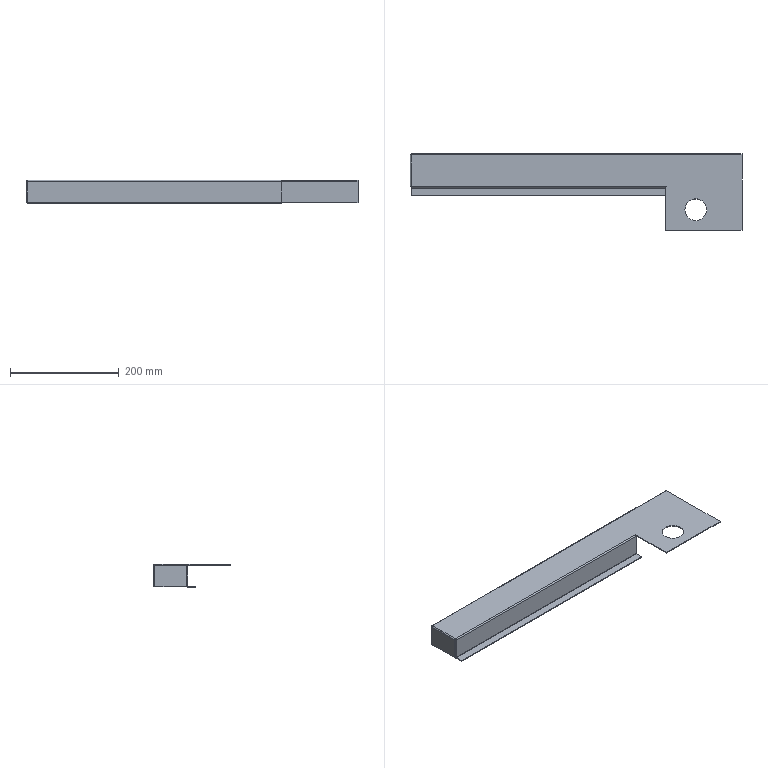Part | NX | 1 solid | 45 faces | box 611.5 x 141.5 x 43 mm | volume 150678 mm3 | plane 32 | cylinder 9 | spline 4 | commonest cylinder face diameters 1.473 x4 4.473 x4 40 x1
STEP:
#1=CARTESIAN_POINT('',(165.,-31.5,-2.237));
#2=VERTEX_POINT('',#1);
#3=CARTESIAN_POINT('',(165.,-31.5,-40.763));
#4=VERTEX_POINT('',#3);
#5=CARTESIAN_POINT('',(165.,-31.5,-41.5));
#6=DIRECTION('',(0.,0.,-1.));
#7=VECTOR('',#6,1000.);
#8=LINE('',#5,#7);
#9=EDGE_CURVE('',#2,#4,#8,.T.);
#10=ORIENTED_EDGE('',*,*,#9,.T.);
#11=CARTESIAN_POINT('',(165.,-30.,-40.763));
#12=VERTEX_POINT('',#11);
#13=CARTESIAN_POINT('',(165.,-31.5,-40.763));
#14=DIRECTION('',(0.,1.,0.));
#15=VECTOR('',#14,1000.);
#16=LINE('',#13,#15);
#17=EDGE_CURVE('',#4,#12,#16,.T.);
#18=ORIENTED_EDGE('',*,*,#17,.T.);
#19=CARTESIAN_POINT('',(165.,-30.,-2.237));
#20=VERTEX_POINT('',#19);
#21=CARTESIAN_POINT('',(165.,-30.,-41.5));
#22=DIRECTION('',(0.,0.,-1.));
#23=VECTOR('',#22,1000.);
#24=LINE('',#21,#23);
#25=EDGE_CURVE('',#20,#12,#24,.T.);
#26=ORIENTED_EDGE('',*,*,#25,.F.);
#27=CARTESIAN_POINT('',(165.,-30.,-2.237));
#28=DIRECTION('',(0.,-1.,0.));
#29=VECTOR('',#28,1000.);
#30=LINE('',#27,#29);
#31=EDGE_CURVE('',#20,#2,#30,.T.);
#32=ORIENTED_EDGE('',*,*,#31,.T.);
#33=EDGE_LOOP('',(#10,#18,#26,#32));
#34=FACE_BOUND('',#33,.T.);
#35=CARTESIAN_POINT('',(165.,-31.5,-41.5));
#36=DIRECTION('',(1.,0.,0.));
#37=DIRECTION('',(0.,1.,0.));
#38=AXIS2_PLACEMENT_3D('',#35,#36,#37);
#39=PLANE('',#38);
#40=ADVANCED_FACE('',(#34),#39,.T.);
#41=CARTESIAN_POINT('',(-304.293,-31.5,-40.763));
#42=VERTEX_POINT('',#41);
#43=CARTESIAN_POINT('',(-304.293,-31.5,-2.237));
#44=VERTEX_POINT('',#43);
#45=CARTESIAN_POINT('',(-304.293,-31.5,0.));
#46=DIRECTION('',(0.,0.,1.));
#47=VECTOR('',#46,1000.);
#48=LINE('',#45,#47);
#49=EDGE_CURVE('',#42,#44,#48,.T.);
#50=ORIENTED_EDGE('',*,*,#49,.F.);
#51=CARTESIAN_POINT('',(165.,-31.5,-40.763));
#52=DIRECTION('',(1.,0.,0.));
#53=VECTOR('',#52,1000.);
#54=LINE('',#51,#53);
#55=EDGE_CURVE('',#4,#42,#54,.F.);
#56=ORIENTED_EDGE('',*,*,#55,.F.);
#57=ORIENTED_EDGE('',*,*,#9,.F.);
#58=CARTESIAN_POINT('',(0.,-31.5,-2.237));
#59=DIRECTION('',(-1.,0.,0.));
#60=VECTOR('',#59,1000.);
#61=LINE('',#58,#60);
#62=EDGE_CURVE('',#2,#44,#61,.T.);
#63=ORIENTED_EDGE('',*,*,#62,.T.);
#64=EDGE_LOOP('',(#50,#56,#57,#63));
#65=FACE_BOUND('',#64,.T.);
#66=CARTESIAN_POINT('',(0.,-31.5,0.));
#67=DIRECTION('',(0.,-1.,0.));
#68=DIRECTION('',(0.,0.,-1.));
#69=AXIS2_PLACEMENT_3D('',#66,#67,#68);
#70=PLANE('',#69);
#71=ADVANCED_FACE('',(#65),#70,.T.);
#72=CARTESIAN_POINT('',(-304.293,-30.,-40.763));
#73=VERTEX_POINT('',#72);
#74=CARTESIAN_POINT('',(165.,-30.,-40.763));
#75=DIRECTION('',(1.,0.,0.));
#76=VECTOR('',#75,1000.);
#77=LINE('',#74,#76);
#78=EDGE_CURVE('',#12,#73,#77,.F.);
#79=ORIENTED_EDGE('',*,*,#78,.T.);
#80=CARTESIAN_POINT('',(-304.293,-30.,-2.237));
#81=VERTEX_POINT('',#80);
#82=CARTESIAN_POINT('',(-304.293,-30.,-1.5));
#83=DIRECTION('',(0.,0.,-1.));
#84=VECTOR('',#83,1000.);
#85=LINE('',#82,#84);
#86=EDGE_CURVE('',#81,#73,#85,.T.);
#87=ORIENTED_EDGE('',*,*,#86,.F.);
#88=CARTESIAN_POINT('',(165.,-30.,-2.237));
#89=DIRECTION('',(-1.,0.,0.));
#90=VECTOR('',#89,1000.);
#91=LINE('',#88,#90);
#92=EDGE_CURVE('',#20,#81,#91,.T.);
#93=ORIENTED_EDGE('',*,*,#92,.F.);
#94=ORIENTED_EDGE('',*,*,#25,.T.);
#95=EDGE_LOOP('',(#79,#87,#93,#94));
#96=FACE_BOUND('',#95,.T.);
#97=CARTESIAN_POINT('',(0.,-30.,0.));
#98=DIRECTION('',(0.,-1.,0.));
#99=DIRECTION('',(0.,0.,-1.));
#100=AXIS2_PLACEMENT_3D('',#97,#98,#99);
#101=PLANE('',#100);
#102=ADVANCED_FACE('',(#96),#101,.F.);
#103=CARTESIAN_POINT('',(-304.293,-31.5,-40.763));
#104=DIRECTION('',(0.,1.,0.));
#105=VECTOR('',#104,1000.);
#106=LINE('',#103,#105);
#107=EDGE_CURVE('',#42,#73,#106,.T.);
#108=ORIENTED_EDGE('',*,*,#107,.F.);
#109=ORIENTED_EDGE('',*,*,#49,.T.);
#110=CARTESIAN_POINT('',(-304.293,-30.,-2.237));
#111=DIRECTION('',(0.,1.,0.));
#112=VECTOR('',#111,1000.);
#113=LINE('',#110,#112);
#114=EDGE_CURVE('',#44,#81,#113,.T.);
#115=ORIENTED_EDGE('',*,*,#114,.T.);
#116=ORIENTED_EDGE('',*,*,#86,.T.);
#117=EDGE_LOOP('',(#108,#109,#115,#116));
#118=FACE_BOUND('',#117,.T.);
#119=CARTESIAN_POINT('',(-304.293,-30.,-1.5));
#120=DIRECTION('',(1.,0.,0.));
#121=DIRECTION('',(0.,0.,-1.));
#122=AXIS2_PLACEMENT_3D('',#119,#120,#121);
#123=PLANE('',#122);
#124=ADVANCED_FACE('',(#118),#123,.F.);
#125=CARTESIAN_POINT('',(200.,-72.,-1.5));
#126=VERTEX_POINT('',#125);
#127=CARTESIAN_POINT('',(220.,-72.,-1.5));
#128=DIRECTION('',(0.,0.,-1.));
#129=DIRECTION('',(-1.,0.,0.));
#130=AXIS2_PLACEMENT_3D('',#127,#128,#129);
#131=CIRCLE('',#130,20.);
#132=EDGE_CURVE('',#126,#126,#131,.T.);
#133=ORIENTED_EDGE('',*,*,#132,.F.);
#134=EDGE_LOOP('',(#133));
#135=FACE_BOUND('',#134,.T.);
#136=CARTESIAN_POINT('',(-304.263,29.263,-1.5));
#137=VERTEX_POINT('',#136);
#138=CARTESIAN_POINT('',(-304.263,-29.263,-1.5));
#139=VERTEX_POINT('',#138);
#140=CARTESIAN_POINT('',(-304.263,29.293,-1.5));
#141=DIRECTION('',(0.,1.,0.));
#142=VECTOR('',#141,1000.);
#143=LINE('',#140,#142);
#144=EDGE_CURVE('',#137,#139,#143,.F.);
#145=ORIENTED_EDGE('',*,*,#144,.F.);
#146=CARTESIAN_POINT('',(305.,29.263,-1.5));
#147=VERTEX_POINT('',#146);
#148=CARTESIAN_POINT('',(305.,29.263,-1.5));
#149=DIRECTION('',(1.,0.,0.));
#150=VECTOR('',#149,1000.);
#151=LINE('',#148,#150);
#152=EDGE_CURVE('',#147,#137,#151,.F.);
#153=ORIENTED_EDGE('',*,*,#152,.F.);
#154=CARTESIAN_POINT('',(305.,-110.,-1.5));
#155=VERTEX_POINT('',#154);
#156=CARTESIAN_POINT('',(305.,-30.,-1.5));
#157=DIRECTION('',(0.,1.,0.));
#158=VECTOR('',#157,1000.);
#159=LINE('',#156,#158);
#160=EDGE_CURVE('',#155,#147,#159,.T.);
#161=ORIENTED_EDGE('',*,*,#160,.F.);
#162=CARTESIAN_POINT('',(165.,-110.,-1.5));
#163=VERTEX_POINT('',#162);
#164=CARTESIAN_POINT('',(305.,-110.,-1.5));
#165=DIRECTION('',(1.,0.,0.));
#166=VECTOR('',#165,1000.);
#167=LINE('',#164,#166);
#168=EDGE_CURVE('',#163,#155,#167,.T.);
#169=ORIENTED_EDGE('',*,*,#168,.F.);
#170=CARTESIAN_POINT('',(165.,-30.,-1.5));
#171=VERTEX_POINT('',#170);
#172=CARTESIAN_POINT('',(165.,-30.,-1.5));
#173=DIRECTION('',(0.,-1.,0.));
#174=VECTOR('',#173,1000.);
#175=LINE('',#172,#174);
#176=EDGE_CURVE('',#171,#163,#175,.T.);
#177=ORIENTED_EDGE('',*,*,#176,.F.);
#178=CARTESIAN_POINT('',(165.75,-30.,-1.5));
#179=VERTEX_POINT('',#178);
#180=CARTESIAN_POINT('',(165.75,-30.,-1.5));
#181=DIRECTION('',(-1.,0.,0.));
#182=VECTOR('',#181,1000.);
#183=LINE('',#180,#182);
#184=EDGE_CURVE('',#179,#171,#183,.T.);
#185=ORIENTED_EDGE('',*,*,#184,.F.);
#186=CARTESIAN_POINT('',(165.75,-28.513,-1.5));
#187=VERTEX_POINT('',#186);
#188=CARTESIAN_POINT('',(165.75,-28.513,-1.5));
#189=DIRECTION('',(0.,-1.,0.));
#190=VECTOR('',#189,1000.);
#191=LINE('',#188,#190);
#192=EDGE_CURVE('',#187,#179,#191,.T.);
#193=ORIENTED_EDGE('',*,*,#192,.F.);
#194=CARTESIAN_POINT('',(165.,-28.513,-1.5));
#195=VERTEX_POINT('',#194);
#196=CARTESIAN_POINT('',(165.,-28.513,-1.5));
#197=DIRECTION('',(1.,0.,0.));
#198=VECTOR('',#197,1000.);
#199=LINE('',#196,#198);
#200=EDGE_CURVE('',#195,#187,#199,.T.);
#201=ORIENTED_EDGE('',*,*,#200,.F.);
#202=CARTESIAN_POINT('',(165.,-29.263,-1.5));
#203=VERTEX_POINT('',#202);
#204=CARTESIAN_POINT('',(165.,-29.263,-1.5));
#205=DIRECTION('',(0.,1.,0.));
#206=VECTOR('',#205,1000.);
#207=LINE('',#204,#206);
#208=EDGE_CURVE('',#203,#195,#207,.T.);
#209=ORIENTED_EDGE('',*,*,#208,.F.);
#210=CARTESIAN_POINT('',(-304.293,-29.263,-1.5));
#211=DIRECTION('',(-1.,0.,0.));
#212=VECTOR('',#211,1000.);
#213=LINE('',#210,#212);
#214=EDGE_CURVE('',#139,#203,#213,.F.);
#215=ORIENTED_EDGE('',*,*,#214,.F.);
#216=EDGE_LOOP('',(#145,#153,#161,#169,#177,#185,#193,#201,#209,#215));
#217=FACE_BOUND('',#216,.T.);
#218=CARTESIAN_POINT('',(0.,0.,-1.5));
#219=DIRECTION('',(0.,0.,-1.));
#220=DIRECTION('',(-1.,0.,0.));
#221=AXIS2_PLACEMENT_3D('',#218,#219,#220);
#222=PLANE('',#221);
#223=ADVANCED_FACE('',(#135,#217),#222,.T.);
#224=CARTESIAN_POINT('',(240.,-72.,0.));
#225=VERTEX_POINT('',#224);
#226=CARTESIAN_POINT('',(220.,-72.,0.));
#227=DIRECTION('',(0.,0.,1.));
#228=DIRECTION('',(1.,0.,0.));
#229=AXIS2_PLACEMENT_3D('',#226,#227,#228);
#230=CIRCLE('',#229,20.);
#231=EDGE_CURVE('',#225,#225,#230,.T.);
#232=ORIENTED_EDGE('',*,*,#231,.F.);
#233=EDGE_LOOP('',(#232));
#234=FACE_BOUND('',#233,.T.);
#235=CARTESIAN_POINT('',(305.,29.263,0.));
#236=VERTEX_POINT('',#235);
#237=CARTESIAN_POINT('',(-304.263,29.263,0.));
#238=VERTEX_POINT('',#237);
#239=CARTESIAN_POINT('',(305.,29.263,0.));
#240=DIRECTION('',(1.,0.,0.));
#241=VECTOR('',#240,1000.);
#242=LINE('',#239,#241);
#243=EDGE_CURVE('',#236,#238,#242,.F.);
#244=ORIENTED_EDGE('',*,*,#243,.T.);
#245=CARTESIAN_POINT('',(-304.263,-29.263,0.));
#246=VERTEX_POINT('',#245);
#247=CARTESIAN_POINT('',(-304.263,29.293,0.));
#248=DIRECTION('',(0.,1.,0.));
#249=VECTOR('',#248,1000.);
#250=LINE('',#247,#249);
#251=EDGE_CURVE('',#238,#246,#250,.F.);
#252=ORIENTED_EDGE('',*,*,#251,.T.);
#253=CARTESIAN_POINT('',(165.,-29.263,0.));
#254=VERTEX_POINT('',#253);
#255=CARTESIAN_POINT('',(-304.293,-29.263,0.));
#256=DIRECTION('',(-1.,0.,0.));
#257=VECTOR('',#256,1000.);
#258=LINE('',#255,#257);
#259=EDGE_CURVE('',#246,#254,#258,.F.);
#260=ORIENTED_EDGE('',*,*,#259,.T.);
#261=CARTESIAN_POINT('',(165.,-28.513,0.));
#262=VERTEX_POINT('',#261);
#263=CARTESIAN_POINT('',(165.,0.,0.));
#264=DIRECTION('',(0.,-1.,0.));
#265=VECTOR('',#264,1000.);
#266=LINE('',#263,#265);
#267=EDGE_CURVE('',#262,#254,#266,.T.);
#268=ORIENTED_EDGE('',*,*,#267,.F.);
#269=CARTESIAN_POINT('',(165.75,-28.513,0.));
#270=VERTEX_POINT('',#269);
#271=CARTESIAN_POINT('',(0.,-28.513,0.));
#272=DIRECTION('',(-1.,0.,0.));
#273=VECTOR('',#272,1000.);
#274=LINE('',#271,#273);
#275=EDGE_CURVE('',#270,#262,#274,.T.);
#276=ORIENTED_EDGE('',*,*,#275,.F.);
#277=CARTESIAN_POINT('',(165.75,-30.,0.));
#278=VERTEX_POINT('',#277);
#279=CARTESIAN_POINT('',(165.75,0.,0.));
#280=DIRECTION('',(0.,1.,0.));
#281=VECTOR('',#280,1000.);
#282=LINE('',#279,#281);
#283=EDGE_CURVE('',#278,#270,#282,.T.);
#284=ORIENTED_EDGE('',*,*,#283,.F.);
#285=CARTESIAN_POINT('',(165.,-30.,0.));
#286=VERTEX_POINT('',#285);
#287=CARTESIAN_POINT('',(0.,-30.,0.));
#288=DIRECTION('',(1.,0.,0.));
#289=VECTOR('',#288,1000.);
#290=LINE('',#287,#289);
#291=EDGE_CURVE('',#286,#278,#290,.T.);
#292=ORIENTED_EDGE('',*,*,#291,.F.);
#293=CARTESIAN_POINT('',(165.,-110.,0.));
#294=VERTEX_POINT('',#293);
#295=CARTESIAN_POINT('',(165.,-30.,0.));
#296=DIRECTION('',(0.,-1.,0.));
#297=VECTOR('',#296,1000.);
#298=LINE('',#295,#297);
#299=EDGE_CURVE('',#286,#294,#298,.T.);
#300=ORIENTED_EDGE('',*,*,#299,.T.);
#301=CARTESIAN_POINT('',(305.,-110.,0.));
#302=VERTEX_POINT('',#301);
#303=CARTESIAN_POINT('',(305.,-110.,0.));
#304=DIRECTION('',(1.,0.,0.));
#305=VECTOR('',#304,1000.);
#306=LINE('',#303,#305);
#307=EDGE_CURVE('',#294,#302,#306,.T.);
#308=ORIENTED_EDGE('',*,*,#307,.T.);
#309=CARTESIAN_POINT('',(305.,-30.,0.));
#310=DIRECTION('',(0.,1.,0.));
#311=VECTOR('',#310,1000.);
#312=LINE('',#309,#311);
#313=EDGE_CURVE('',#302,#236,#312,.T.);
#314=ORIENTED_EDGE('',*,*,#313,.T.);
#315=EDGE_LOOP('',(#244,#252,#260,#268,#276,#284,#292,#300,#308,#314));
#316=FACE_BOUND('',#315,.T.);
#317=CARTESIAN_POINT('',(0.,0.,0.));
#318=DIRECTION('',(0.,0.,-1.));
#319=DIRECTION('',(-1.,0.,0.));
#320=AXIS2_PLACEMENT_3D('',#317,#318,#319);
#321=PLANE('',#320);
#322=ADVANCED_FACE('',(#234,#316),#321,.F.);
#323=ORIENTED_EDGE('',*,*,#160,.T.);
#324=CARTESIAN_POINT('',(305.,29.263,-1.5));
#325=DIRECTION('',(0.,0.,1.));
#326=VECTOR('',#325,1000.);
#327=LINE('',#324,#326);
#328=EDGE_CURVE('',#147,#236,#327,.T.);
#329=ORIENTED_EDGE('',*,*,#328,.T.);
#330=ORIENTED_EDGE('',*,*,#313,.F.);
#331=CARTESIAN_POINT('',(305.,-110.,-1.5));
#332=DIRECTION('',(0.,0.,1.));
#333=VECTOR('',#332,1000.);
#334=LINE('',#331,#333);
#335=EDGE_CURVE('',#155,#302,#334,.T.);
#336=ORIENTED_EDGE('',*,*,#335,.F.);
#337=EDGE_LOOP('',(#323,#329,#330,#336));
#338=FACE_BOUND('',#337,.T.);
#339=CARTESIAN_POINT('',(305.,-30.,-1.5));
#340=DIRECTION('',(1.,0.,0.));
#341=DIRECTION('',(0.,0.,-1.));
#342=AXIS2_PLACEMENT_3D('',#339,#340,#341);
#343=PLANE('',#342);
#344=ADVANCED_FACE('',(#338),#343,.T.);
#345=ORIENTED_EDGE('',*,*,#307,.F.);
#346=CARTESIAN_POINT('',(165.,-110.,-1.5));
#347=DIRECTION('',(0.,0.,1.));
#348=VECTOR('',#347,1000.);
#349=LINE('',#346,#348);
#350=EDGE_CURVE('',#163,#294,#349,.T.);
#351=ORIENTED_EDGE('',*,*,#350,.F.);
#352=ORIENTED_EDGE('',*,*,#168,.T.);
#353=ORIENTED_EDGE('',*,*,#335,.T.);
#354=EDGE_LOOP('',(#345,#351,#352,#353));
#355=FACE_BOUND('',#354,.T.);
#356=CARTESIAN_POINT('',(305.,-110.,-1.5));
#357=DIRECTION('',(0.,-1.,0.));
#358=DIRECTION('',(1.,0.,0.));
#359=AXIS2_PLACEMENT_3D('',#356,#357,#358);
#360=PLANE('',#359);
#361=ADVANCED_FACE('',(#355),#360,.T.);
#362=ORIENTED_EDGE('',*,*,#299,.F.);
#363=CARTESIAN_POINT('',(165.,-30.,-1.5));
#364=DIRECTION('',(0.,0.,1.));
#365=VECTOR('',#364,1000.);
#366=LINE('',#363,#365);
#367=EDGE_CURVE('',#171,#286,#366,.T.);
#368=ORIENTED_EDGE('',*,*,#367,.F.);
#369=ORIENTED_EDGE('',*,*,#176,.T.);
#370=ORIENTED_EDGE('',*,*,#350,.T.);
#371=EDGE_LOOP('',(#362,#368,#369,#370));
#372=FACE_BOUND('',#371,.T.);
#373=CARTESIAN_POINT('',(165.,-30.,-1.5));
#374=DIRECTION('',(-1.,0.,0.));
#375=DIRECTION('',(0.,0.,1.));
#376=AXIS2_PLACEMENT_3D('',#373,#374,#375);
#377=PLANE('',#376);
#378=ADVANCED_FACE('',(#372),#377,.T.);
#379=CARTESIAN_POINT('',(165.,-28.513,-1.5));
#380=DIRECTION('',(0.,0.,1.));
#381=VECTOR('',#380,1000.);
#382=LINE('',#379,#381);
#383=EDGE_CURVE('',#195,#262,#382,.T.);
#384=ORIENTED_EDGE('',*,*,#383,.T.);
#385=ORIENTED_EDGE('',*,*,#267,.T.);
#386=CARTESIAN_POINT('',(165.,-29.263,-1.5));
#387=DIRECTION('',(0.,0.,1.));
#388=VECTOR('',#387,1000.);
#389=LINE('',#386,#388);
#390=EDGE_CURVE('',#203,#254,#389,.T.);
#391=ORIENTED_EDGE('',*,*,#390,.F.);
#392=ORIENTED_EDGE('',*,*,#208,.T.);
#393=EDGE_LOOP('',(#384,#385,#391,#392));
#394=FACE_BOUND('',#393,.T.);
#395=CARTESIAN_POINT('',(165.,-29.263,-1.5));
#396=DIRECTION('',(1.,0.,0.));
#397=DIRECTION('',(0.,0.,-1.));
#398=AXIS2_PLACEMENT_3D('',#395,#396,#397);
#399=PLANE('',#398);
#400=ADVANCED_FACE('',(#394),#399,.T.);
#401=CARTESIAN_POINT('',(165.75,-28.513,-1.5));
#402=DIRECTION('',(0.,0.,1.));
#403=VECTOR('',#402,1000.);
#404=LINE('',#401,#403);
#405=EDGE_CURVE('',#187,#270,#404,.T.);
#406=ORIENTED_EDGE('',*,*,#405,.T.);
#407=ORIENTED_EDGE('',*,*,#275,.T.);
#408=ORIENTED_EDGE('',*,*,#383,.F.);
#409=ORIENTED_EDGE('',*,*,#200,.T.);
#410=EDGE_LOOP('',(#406,#407,#408,#409));
#411=FACE_BOUND('',#410,.T.);
#412=CARTESIAN_POINT('',(165.,-28.513,-1.5));
#413=DIRECTION('',(0.,-1.,0.));
#414=DIRECTION('',(0.,0.,-1.));
#415=AXIS2_PLACEMENT_3D('',#412,#413,#414);
#416=PLANE('',#415);
#417=ADVANCED_FACE('',(#411),#416,.T.);
#418=CARTESIAN_POINT('',(165.75,-30.,-1.5));
#419=DIRECTION('',(0.,0.,1.));
#420=VECTOR('',#419,1000.);
#421=LINE('',#418,#420);
#422=EDGE_CURVE('',#179,#278,#421,.T.);
#423=ORIENTED_EDGE('',*,*,#422,.T.);
#424=ORIENTED_EDGE('',*,*,#283,.T.);
#425=ORIENTED_EDGE('',*,*,#405,.F.);
#426=ORIENTED_EDGE('',*,*,#192,.T.);
#427=EDGE_LOOP('',(#423,#424,#425,#426));
#428=FACE_BOUND('',#427,.T.);
#429=CARTESIAN_POINT('',(165.75,-28.513,-1.5));
#430=DIRECTION('',(-1.,0.,0.));
#431=DIRECTION('',(0.,0.,1.));
#432=AXIS2_PLACEMENT_3D('',#429,#430,#431);
#433=PLANE('',#432);
#434=ADVANCED_FACE('',(#428),#433,.T.);
#435=ORIENTED_EDGE('',*,*,#367,.T.);
#436=ORIENTED_EDGE('',*,*,#291,.T.);
#437=ORIENTED_EDGE('',*,*,#422,.F.);
#438=ORIENTED_EDGE('',*,*,#184,.T.);
#439=EDGE_LOOP('',(#435,#436,#437,#438));
#440=FACE_BOUND('',#439,.T.);
#441=CARTESIAN_POINT('',(165.75,-30.,-1.5));
#442=DIRECTION('',(0.,1.,0.));
#443=DIRECTION('',(0.,0.,1.));
#444=AXIS2_PLACEMENT_3D('',#441,#442,#443);
#445=PLANE('',#444);
#446=ADVANCED_FACE('',(#440),#445,.T.);
#447=ORIENTED_EDGE('',*,*,#31,.F.);
#448=CARTESIAN_POINT('',(165.,-29.263,-2.237));
#449=DIRECTION('',(-1.,0.,0.));
#450=DIRECTION('',(0.,0.,1.));
#451=AXIS2_PLACEMENT_3D('',#448,#449,#450);
#452=CIRCLE('',#451,0.7366);
#453=EDGE_CURVE('',#203,#20,#452,.F.);
#454=ORIENTED_EDGE('',*,*,#453,.F.);
#455=ORIENTED_EDGE('',*,*,#390,.T.);
#456=CARTESIAN_POINT('',(165.,-29.263,-2.237));
#457=DIRECTION('',(-1.,0.,0.));
#458=DIRECTION('',(0.,0.,1.));
#459=AXIS2_PLACEMENT_3D('',#456,#457,#458);
#460=CIRCLE('',#459,2.237);
#461=EDGE_CURVE('',#254,#2,#460,.F.);
#462=ORIENTED_EDGE('',*,*,#461,.T.);
#463=EDGE_LOOP('',(#447,#454,#455,#462));
#464=FACE_BOUND('',#463,.T.);
#465=CARTESIAN_POINT('',(165.,-29.263,-2.237));
#466=DIRECTION('',(1.,0.,0.));
#467=DIRECTION('',(0.,0.,-1.));
#468=AXIS2_PLACEMENT_3D('',#465,#466,#467);
#469=PLANE('',#468);
#470=ADVANCED_FACE('',(#464),#469,.T.);
#471=CARTESIAN_POINT('',(-304.293,-30.,-2.237));
#472=CARTESIAN_POINT('',(-304.283,-30.,-1.851));
#473=CARTESIAN_POINT('',(-304.273,-29.649,-1.5));
#474=CARTESIAN_POINT('',(-304.263,-29.263,-1.5));
#475=B_SPLINE_CURVE_WITH_KNOTS('',3,(#471,#472,#473,#474),.UNSPECIFIED.,.F.,.F.,(4,4),(0.,1.),.UNSPECIFIED.);
#476=EDGE_CURVE('',#81,#139,#475,.T.);
#477=ORIENTED_EDGE('',*,*,#476,.F.);
#478=ORIENTED_EDGE('',*,*,#114,.F.);
#479=CARTESIAN_POINT('',(-304.293,-31.5,-2.237));
#480=CARTESIAN_POINT('',(-304.288,-31.5,-1.651));
#481=CARTESIAN_POINT('',(-304.278,-31.015,-0.4846));
#482=CARTESIAN_POINT('',(-304.268,-29.849,0.));
#483=CARTESIAN_POINT('',(-304.263,-29.263,0.));
#484=B_SPLINE_CURVE_WITH_KNOTS('',3,(#479,#480,#481,#482,#483),.UNSPECIFIED.,.F.,.F.,(4,1,4),(0.,0.5,1.),.UNSPECIFIED.);
#485=EDGE_CURVE('',#44,#246,#484,.T.);
#486=ORIENTED_EDGE('',*,*,#485,.T.);
#487=CARTESIAN_POINT('',(-304.263,-29.263,-1.5));
#488=DIRECTION('',(0.,0.,1.));
#489=VECTOR('',#488,1000.);
#490=LINE('',#487,#489);
#491=EDGE_CURVE('',#139,#246,#490,.T.);
#492=ORIENTED_EDGE('',*,*,#491,.F.);
#493=EDGE_LOOP('',(#477,#478,#486,#492));
#494=FACE_BOUND('',#493,.T.);
#495=CARTESIAN_POINT('',(-304.293,-31.515,-2.237));
#496=CARTESIAN_POINT('',(-304.29,-31.515,-1.942));
#497=CARTESIAN_POINT('',(-304.288,-31.456,-1.647));
#498=CARTESIAN_POINT('',(-304.283,-31.231,-1.103));
#499=CARTESIAN_POINT('',(-304.281,-31.064,-0.8529));
#500=CARTESIAN_POINT('',(-304.276,-30.647,-0.4361));
#501=CARTESIAN_POINT('',(-304.273,-30.397,-0.2692));
#502=CARTESIAN_POINT('',(-304.268,-29.853,-0.0436));
#503=CARTESIAN_POINT('',(-304.266,-29.558,0.015));
#504=CARTESIAN_POINT('',(-304.263,-29.263,0.015));
#505=CARTESIAN_POINT('',(-304.293,-31.5,-2.237));
#506=CARTESIAN_POINT('',(-304.29,-31.5,-1.944));
#507=CARTESIAN_POINT('',(-304.288,-31.442,-1.651));
#508=CARTESIAN_POINT('',(-304.283,-31.218,-1.11));
#509=CARTESIAN_POINT('',(-304.281,-31.052,-0.8621));
#510=CARTESIAN_POINT('',(-304.276,-30.638,-0.4481));
#511=CARTESIAN_POINT('',(-304.273,-30.39,-0.2823));
#512=CARTESIAN_POINT('',(-304.268,-29.849,-0.05821));
#513=CARTESIAN_POINT('',(-304.266,-29.556,0.));
#514=CARTESIAN_POINT('',(-304.263,-29.263,0.));
#515=CARTESIAN_POINT('',(-304.293,-30.,-2.237));
#516=CARTESIAN_POINT('',(-304.29,-30.,-2.14));
#517=CARTESIAN_POINT('',(-304.288,-29.981,-2.044));
#518=CARTESIAN_POINT('',(-304.283,-29.907,-1.866));
#519=CARTESIAN_POINT('',(-304.281,-29.852,-1.784));
#520=CARTESIAN_POINT('',(-304.276,-29.716,-1.648));
#521=CARTESIAN_POINT('',(-304.273,-29.634,-1.593));
#522=CARTESIAN_POINT('',(-304.268,-29.456,-1.519));
#523=CARTESIAN_POINT('',(-304.266,-29.36,-1.5));
#524=CARTESIAN_POINT('',(-304.263,-29.263,-1.5));
#525=CARTESIAN_POINT('',(-304.293,-29.985,-2.237));
#526=CARTESIAN_POINT('',(-304.29,-29.985,-2.142));
#527=CARTESIAN_POINT('',(-304.288,-29.966,-2.048));
#528=CARTESIAN_POINT('',(-304.283,-29.894,-1.873));
#529=CARTESIAN_POINT('',(-304.281,-29.84,-1.793));
#530=CARTESIAN_POINT('',(-304.276,-29.707,-1.66));
#531=CARTESIAN_POINT('',(-304.273,-29.627,-1.606));
#532=CARTESIAN_POINT('',(-304.268,-29.452,-1.534));
#533=CARTESIAN_POINT('',(-304.266,-29.358,-1.515));
#534=CARTESIAN_POINT('',(-304.263,-29.263,-1.515));
#535=B_SPLINE_SURFACE_WITH_KNOTS('',1,3,((#495,#496,#497,#498,#499,#500,#501,#502,#503,#504),(#505,#506,#507,#508,#509,#510,#511,#512,#513,#514),(#515,#516,#517,#518,#519,#520,#521,#522,#523,#524),(#525,#526,#527,#528,#529,#530,#531,#532,#533,#534)),.RULED_SURF.,.F.,.F.,.F.,(2,1,1,2),(4,2,2,2,4),(-0.01,0.,1.,1.01),(0.,0.25,0.5,0.75,1.),.UNSPECIFIED.);
#536=ADVANCED_FACE('',(#494),#535,.F.);
#537=ORIENTED_EDGE('',*,*,#259,.F.);
#538=ORIENTED_EDGE('',*,*,#485,.F.);
#539=ORIENTED_EDGE('',*,*,#62,.F.);
#540=ORIENTED_EDGE('',*,*,#461,.F.);
#541=EDGE_LOOP('',(#537,#538,#539,#540));
#542=FACE_BOUND('',#541,.T.);
#543=CARTESIAN_POINT('',(-304.293,-29.263,-2.237));
#544=DIRECTION('',(-1.,0.,0.));
#545=DIRECTION('',(0.,-1.,0.));
#546=AXIS2_PLACEMENT_3D('',#543,#544,#545);
#547=CYLINDRICAL_SURFACE('',#546,2.237);
#548=ADVANCED_FACE('',(#542),#547,.T.);
#549=ORIENTED_EDGE('',*,*,#214,.T.);
#550=ORIENTED_EDGE('',*,*,#453,.T.);
#551=ORIENTED_EDGE('',*,*,#92,.T.);
#552=ORIENTED_EDGE('',*,*,#476,.T.);
#553=EDGE_LOOP('',(#549,#550,#551,#552));
#554=FACE_BOUND('',#553,.T.);
#555=CARTESIAN_POINT('',(-304.293,-29.263,-2.237));
#556=DIRECTION('',(-1.,0.,0.));
#557=DIRECTION('',(0.,-1.,0.));
#558=AXIS2_PLACEMENT_3D('',#555,#556,#557);
#559=CYLINDRICAL_SURFACE('',#558,0.7366);
#560=ADVANCED_FACE('',(#554),#559,.F.);
#561=CARTESIAN_POINT('',(-306.5,-29.293,-2.237));
#562=VERTEX_POINT('',#561);
#563=CARTESIAN_POINT('',(-305.,-29.293,-2.237));
#564=VERTEX_POINT('',#563);
#565=CARTESIAN_POINT('',(-305.,-29.293,-2.237));
#566=DIRECTION('',(1.,0.,0.));
#567=VECTOR('',#566,1000.);
#568=LINE('',#565,#567);
#569=EDGE_CURVE('',#562,#564,#568,.T.);
#570=ORIENTED_EDGE('',*,*,#569,.T.);
#571=CARTESIAN_POINT('',(-304.263,-29.263,-1.5));
#572=CARTESIAN_POINT('',(-304.649,-29.273,-1.5));
#573=CARTESIAN_POINT('',(-305.,-29.283,-1.851));
#574=CARTESIAN_POINT('',(-305.,-29.293,-2.237));
#575=B_SPLINE_CURVE_WITH_KNOTS('',3,(#571,#572,#573,#574),.UNSPECIFIED.,.F.,.F.,(4,4),(0.,1.),.UNSPECIFIED.);
#576=EDGE_CURVE('',#139,#564,#575,.T.);
#577=ORIENTED_EDGE('',*,*,#576,.F.);
#578=ORIENTED_EDGE('',*,*,#491,.T.);
#579=CARTESIAN_POINT('',(-304.263,-29.263,0.));
#580=CARTESIAN_POINT('',(-304.849,-29.268,0.));
#581=CARTESIAN_POINT('',(-306.015,-29.278,-0.4846));
#582=CARTESIAN_POINT('',(-306.5,-29.288,-1.651));
#583=CARTESIAN_POINT('',(-306.5,-29.293,-2.237));
#584=B_SPLINE_CURVE_WITH_KNOTS('',3,(#579,#580,#581,#582,#583),.UNSPECIFIED.,.F.,.F.,(4,1,4),(0.,0.5,1.),.UNSPECIFIED.);
#585=EDGE_CURVE('',#246,#562,#584,.T.);
#586=ORIENTED_EDGE('',*,*,#585,.T.);
#587=EDGE_LOOP('',(#570,#577,#578,#586));
#588=FACE_BOUND('',#587,.T.);
#589=CARTESIAN_POINT('',(-304.263,-29.263,0.015));
#590=CARTESIAN_POINT('',(-304.558,-29.266,0.015));
#591=CARTESIAN_POINT('',(-304.853,-29.268,-0.0436));
#592=CARTESIAN_POINT('',(-305.397,-29.273,-0.2692));
#593=CARTESIAN_POINT('',(-305.647,-29.276,-0.4361));
#594=CARTESIAN_POINT('',(-306.064,-29.281,-0.8529));
#595=CARTESIAN_POINT('',(-306.231,-29.283,-1.103));
#596=CARTESIAN_POINT('',(-306.456,-29.288,-1.647));
#597=CARTESIAN_POINT('',(-306.515,-29.29,-1.942));
#598=CARTESIAN_POINT('',(-306.515,-29.293,-2.237));
#599=CARTESIAN_POINT('',(-304.263,-29.263,0.));
#600=CARTESIAN_POINT('',(-304.556,-29.266,0.));
#601=CARTESIAN_POINT('',(-304.849,-29.268,-0.05821));
#602=CARTESIAN_POINT('',(-305.39,-29.273,-0.2823));
#603=CARTESIAN_POINT('',(-305.638,-29.276,-0.4481));
#604=CARTESIAN_POINT('',(-306.052,-29.281,-0.8621));
#605=CARTESIAN_POINT('',(-306.218,-29.283,-1.11));
#606=CARTESIAN_POINT('',(-306.442,-29.288,-1.651));
#607=CARTESIAN_POINT('',(-306.5,-29.29,-1.944));
#608=CARTESIAN_POINT('',(-306.5,-29.293,-2.237));
#609=CARTESIAN_POINT('',(-304.263,-29.263,-1.5));
#610=CARTESIAN_POINT('',(-304.36,-29.266,-1.5));
#611=CARTESIAN_POINT('',(-304.456,-29.268,-1.519));
#612=CARTESIAN_POINT('',(-304.634,-29.273,-1.593));
#613=CARTESIAN_POINT('',(-304.716,-29.276,-1.648));
#614=CARTESIAN_POINT('',(-304.852,-29.281,-1.784));
#615=CARTESIAN_POINT('',(-304.907,-29.283,-1.866));
#616=CARTESIAN_POINT('',(-304.981,-29.288,-2.044));
#617=CARTESIAN_POINT('',(-305.,-29.29,-2.14));
#618=CARTESIAN_POINT('',(-305.,-29.293,-2.237));
#619=CARTESIAN_POINT('',(-304.263,-29.263,-1.515));
#620=CARTESIAN_POINT('',(-304.358,-29.266,-1.515));
#621=CARTESIAN_POINT('',(-304.452,-29.268,-1.534));
#622=CARTESIAN_POINT('',(-304.627,-29.273,-1.606));
#623=CARTESIAN_POINT('',(-304.707,-29.276,-1.66));
#624=CARTESIAN_POINT('',(-304.84,-29.281,-1.793));
#625=CARTESIAN_POINT('',(-304.894,-29.283,-1.873));
#626=CARTESIAN_POINT('',(-304.966,-29.288,-2.048));
#627=CARTESIAN_POINT('',(-304.985,-29.29,-2.142));
#628=CARTESIAN_POINT('',(-304.985,-29.293,-2.237));
#629=B_SPLINE_SURFACE_WITH_KNOTS('',1,3,((#589,#590,#591,#592,#593,#594,#595,#596,#597,#598),(#599,#600,#601,#602,#603,#604,#605,#606,#607,#608),(#609,#610,#611,#612,#613,#614,#615,#616,#617,#618),(#619,#620,#621,#622,#623,#624,#625,#626,#627,#628)),.RULED_SURF.,.F.,.F.,.F.,(2,1,1,2),(4,2,2,2,4),(-0.01,0.,1.,1.01),(0.,0.25,0.5,0.75,1.),.UNSPECIFIED.);
#630=ADVANCED_FACE('',(#588),#629,.F.);
#631=CARTESIAN_POINT('',(-305.,29.293,-2.237));
#632=VERTEX_POINT('',#631);
#633=CARTESIAN_POINT('',(-305.,29.293,-2.237));
#634=CARTESIAN_POINT('',(-305.,29.283,-1.851));
#635=CARTESIAN_POINT('',(-304.649,29.273,-1.5));
#636=CARTESIAN_POINT('',(-304.263,29.263,-1.5));
#637=B_SPLINE_CURVE_WITH_KNOTS('',3,(#633,#634,#635,#636),.UNSPECIFIED.,.F.,.F.,(4,4),(0.,1.),.UNSPECIFIED.);
#638=EDGE_CURVE('',#632,#137,#637,.T.);
#639=ORIENTED_EDGE('',*,*,#638,.F.);
#640=CARTESIAN_POINT('',(-306.5,29.293,-2.237));
#641=VERTEX_POINT('',#640);
#642=CARTESIAN_POINT('',(-305.,29.293,-2.237));
#643=DIRECTION('',(1.,0.,0.));
#644=VECTOR('',#643,1000.);
#645=LINE('',#642,#644);
#646=EDGE_CURVE('',#641,#632,#645,.T.);
#647=ORIENTED_EDGE('',*,*,#646,.F.);
#648=CARTESIAN_POINT('',(-306.5,29.293,-2.237));
#649=CARTESIAN_POINT('',(-306.5,29.288,-1.651));
#650=CARTESIAN_POINT('',(-306.015,29.278,-0.4846));
#651=CARTESIAN_POINT('',(-304.849,29.268,0.));
#652=CARTESIAN_POINT('',(-304.263,29.263,0.));
#653=B_SPLINE_CURVE_WITH_KNOTS('',3,(#648,#649,#650,#651,#652),.UNSPECIFIED.,.F.,.F.,(4,1,4),(0.,0.5,1.),.UNSPECIFIED.);
#654=EDGE_CURVE('',#641,#238,#653,.T.);
#655=ORIENTED_EDGE('',*,*,#654,.T.);
#656=CARTESIAN_POINT('',(-304.263,29.263,-1.5));
#657=DIRECTION('',(0.,0.,1.));
#658=VECTOR('',#657,1000.);
#659=LINE('',#656,#658);
#660=EDGE_CURVE('',#137,#238,#659,.T.);
#661=ORIENTED_EDGE('',*,*,#660,.F.);
#662=EDGE_LOOP('',(#639,#647,#655,#661));
#663=FACE_BOUND('',#662,.T.);
#664=CARTESIAN_POINT('',(-306.515,29.293,-2.237));
#665=CARTESIAN_POINT('',(-306.515,29.29,-1.942));
#666=CARTESIAN_POINT('',(-306.456,29.288,-1.647));
#667=CARTESIAN_POINT('',(-306.231,29.283,-1.103));
#668=CARTESIAN_POINT('',(-306.064,29.281,-0.8529));
#669=CARTESIAN_POINT('',(-305.647,29.276,-0.4361));
#670=CARTESIAN_POINT('',(-305.397,29.273,-0.2692));
#671=CARTESIAN_POINT('',(-304.853,29.268,-0.0436));
#672=CARTESIAN_POINT('',(-304.558,29.266,0.015));
#673=CARTESIAN_POINT('',(-304.263,29.263,0.015));
#674=CARTESIAN_POINT('',(-306.5,29.293,-2.237));
#675=CARTESIAN_POINT('',(-306.5,29.29,-1.944));
#676=CARTESIAN_POINT('',(-306.442,29.288,-1.651));
#677=CARTESIAN_POINT('',(-306.218,29.283,-1.11));
#678=CARTESIAN_POINT('',(-306.052,29.281,-0.8621));
#679=CARTESIAN_POINT('',(-305.638,29.276,-0.4481));
#680=CARTESIAN_POINT('',(-305.39,29.273,-0.2823));
#681=CARTESIAN_POINT('',(-304.849,29.268,-0.05821));
#682=CARTESIAN_POINT('',(-304.556,29.266,0.));
#683=CARTESIAN_POINT('',(-304.263,29.263,0.));
#684=CARTESIAN_POINT('',(-305.,29.293,-2.237));
#685=CARTESIAN_POINT('',(-305.,29.29,-2.14));
#686=CARTESIAN_POINT('',(-304.981,29.288,-2.044));
#687=CARTESIAN_POINT('',(-304.907,29.283,-1.866));
#688=CARTESIAN_POINT('',(-304.852,29.281,-1.784));
#689=CARTESIAN_POINT('',(-304.716,29.276,-1.648));
#690=CARTESIAN_POINT('',(-304.634,29.273,-1.593));
#691=CARTESIAN_POINT('',(-304.456,29.268,-1.519));
#692=CARTESIAN_POINT('',(-304.36,29.266,-1.5));
#693=CARTESIAN_POINT('',(-304.263,29.263,-1.5));
#694=CARTESIAN_POINT('',(-304.985,29.293,-2.237));
#695=CARTESIAN_POINT('',(-304.985,29.29,-2.142));
#696=CARTESIAN_POINT('',(-304.966,29.288,-2.048));
#697=CARTESIAN_POINT('',(-304.894,29.283,-1.873));
#698=CARTESIAN_POINT('',(-304.84,29.281,-1.793));
#699=CARTESIAN_POINT('',(-304.707,29.276,-1.66));
#700=CARTESIAN_POINT('',(-304.627,29.273,-1.606));
#701=CARTESIAN_POINT('',(-304.452,29.268,-1.534));
#702=CARTESIAN_POINT('',(-304.358,29.266,-1.515));
#703=CARTESIAN_POINT('',(-304.263,29.263,-1.515));
#704=B_SPLINE_SURFACE_WITH_KNOTS('',1,3,((#664,#665,#666,#667,#668,#669,#670,#671,#672,#673),(#674,#675,#676,#677,#678,#679,#680,#681,#682,#683),(#684,#685,#686,#687,#688,#689,#690,#691,#692,#693),(#694,#695,#696,#697,#698,#699,#700,#701,#702,#703)),.RULED_SURF.,.F.,.F.,.F.,(2,1,1,2),(4,2,2,2,4),(-0.01,0.,1.,1.01),(0.,0.25,0.5,0.75,1.),.UNSPECIFIED.);
#705=ADVANCED_FACE('',(#663),#704,.F.);
#706=ORIENTED_EDGE('',*,*,#251,.F.);
#707=ORIENTED_EDGE('',*,*,#654,.F.);
#708=CARTESIAN_POINT('',(-306.5,0.,-2.237));
#709=DIRECTION('',(0.,-1.,0.));
#710=VECTOR('',#709,1000.);
#711=LINE('',#708,#710);
#712=EDGE_CURVE('',#641,#562,#711,.T.);
#713=ORIENTED_EDGE('',*,*,#712,.T.);
#714=ORIENTED_EDGE('',*,*,#585,.F.);
#715=EDGE_LOOP('',(#706,#707,#713,#714));
#716=FACE_BOUND('',#715,.T.);
#717=CARTESIAN_POINT('',(-304.263,29.293,-2.237));
#718=DIRECTION('',(0.,1.,0.));
#719=DIRECTION('',(-1.,0.,0.));
#720=AXIS2_PLACEMENT_3D('',#717,#718,#719);
#721=CYLINDRICAL_SURFACE('',#720,2.237);
#722=ADVANCED_FACE('',(#716),#721,.T.);
#723=ORIENTED_EDGE('',*,*,#144,.T.);
#724=ORIENTED_EDGE('',*,*,#576,.T.);
#725=CARTESIAN_POINT('',(-305.,-30.,-2.237));
#726=DIRECTION('',(0.,1.,0.));
#727=VECTOR('',#726,1000.);
#728=LINE('',#725,#727);
#729=EDGE_CURVE('',#564,#632,#728,.T.);
#730=ORIENTED_EDGE('',*,*,#729,.T.);
#731=ORIENTED_EDGE('',*,*,#638,.T.);
#732=EDGE_LOOP('',(#723,#724,#730,#731));
#733=FACE_BOUND('',#732,.T.);
#734=CARTESIAN_POINT('',(-304.263,29.293,-2.237));
#735=DIRECTION('',(0.,1.,0.));
#736=DIRECTION('',(-1.,0.,0.));
#737=AXIS2_PLACEMENT_3D('',#734,#735,#736);
#738=CYLINDRICAL_SURFACE('',#737,0.7366);
#739=ADVANCED_FACE('',(#733),#738,.F.);
#740=CARTESIAN_POINT('',(-305.,-29.293,-41.5));
#741=VERTEX_POINT('',#740);
#742=CARTESIAN_POINT('',(-306.5,-29.293,-41.5));
#743=VERTEX_POINT('',#742);
#744=CARTESIAN_POINT('',(-306.5,-29.293,-41.5));
#745=DIRECTION('',(-1.,0.,0.));
#746=VECTOR('',#745,1000.);
#747=LINE('',#744,#746);
#748=EDGE_CURVE('',#741,#743,#747,.T.);
#749=ORIENTED_EDGE('',*,*,#748,.F.);
#750=CARTESIAN_POINT('',(-305.,-29.293,-1.5));
#751=DIRECTION('',(0.,0.,-1.));
#752=VECTOR('',#751,1000.);
#753=LINE('',#750,#752);
#754=EDGE_CURVE('',#564,#741,#753,.T.);
#755=ORIENTED_EDGE('',*,*,#754,.F.);
#756=ORIENTED_EDGE('',*,*,#569,.F.);
#757=CARTESIAN_POINT('',(-306.5,-29.293,0.));
#758=DIRECTION('',(0.,0.,-1.));
#759=VECTOR('',#758,1000.);
#760=LINE('',#757,#759);
#761=EDGE_CURVE('',#562,#743,#760,.T.);
#762=ORIENTED_EDGE('',*,*,#761,.T.);
#763=EDGE_LOOP('',(#749,#755,#756,#762));
#764=FACE_BOUND('',#763,.T.);
#765=CARTESIAN_POINT('',(-305.,-29.293,-1.5));
#766=DIRECTION('',(0.,-1.,0.));
#767=DIRECTION('',(0.,0.,-1.));
#768=AXIS2_PLACEMENT_3D('',#765,#766,#767);
#769=PLANE('',#768);
#770=ADVANCED_FACE('',(#764),#769,.T.);
#771=ORIENTED_EDGE('',*,*,#712,.F.);
#772=CARTESIAN_POINT('',(-306.5,29.293,-41.5));
#773=VERTEX_POINT('',#772);
#774=CARTESIAN_POINT('',(-306.5,29.293,0.));
#775=DIRECTION('',(0.,0.,-1.));
#776=VECTOR('',#775,1000.);
#777=LINE('',#774,#776);
#778=EDGE_CURVE('',#641,#773,#777,.T.);
#779=ORIENTED_EDGE('',*,*,#778,.T.);
#780=CARTESIAN_POINT('',(-306.5,-30.,-41.5));
#781=DIRECTION('',(0.,1.,0.));
#782=VECTOR('',#781,1000.);
#783=LINE('',#780,#782);
#784=EDGE_CURVE('',#743,#773,#783,.T.);
#785=ORIENTED_EDGE('',*,*,#784,.F.);
#786=ORIENTED_EDGE('',*,*,#761,.F.);
#787=EDGE_LOOP('',(#771,#779,#785,#786));
#788=FACE_BOUND('',#787,.T.);
#789=CARTESIAN_POINT('',(-306.5,0.,0.));
#790=DIRECTION('',(1.,0.,0.));
#791=DIRECTION('',(0.,0.,-1.));
#792=AXIS2_PLACEMENT_3D('',#789,#790,#791);
#793=PLANE('',#792);
#794=ADVANCED_FACE('',(#788),#793,.F.);
#795=CARTESIAN_POINT('',(-305.,29.293,-41.5));
#796=VERTEX_POINT('',#795);
#797=CARTESIAN_POINT('',(-305.,29.293,-1.5));
#798=DIRECTION('',(0.,0.,-1.));
#799=VECTOR('',#798,1000.);
#800=LINE('',#797,#799);
#801=EDGE_CURVE('',#632,#796,#800,.T.);
#802=ORIENTED_EDGE('',*,*,#801,.F.);
#803=ORIENTED_EDGE('',*,*,#729,.F.);
#804=ORIENTED_EDGE('',*,*,#754,.T.);
#805=CARTESIAN_POINT('',(-305.,-30.,-41.5));
#806=DIRECTION('',(0.,1.,0.));
#807=VECTOR('',#806,1000.);
#808=LINE('',#805,#807);
#809=EDGE_CURVE('',#741,#796,#808,.T.);
#810=ORIENTED_EDGE('',*,*,#809,.T.);
#811=EDGE_LOOP('',(#802,#803,#804,#810));
#812=FACE_BOUND('',#811,.T.);
#813=CARTESIAN_POINT('',(-305.,0.,0.));
#814=DIRECTION('',(1.,0.,0.));
#815=DIRECTION('',(0.,0.,-1.));
#816=AXIS2_PLACEMENT_3D('',#813,#814,#815);
#817=PLANE('',#816);
#818=ADVANCED_FACE('',(#812),#817,.T.);
#819=CARTESIAN_POINT('',(-306.5,29.293,-41.5));
#820=DIRECTION('',(-1.,0.,0.));
#821=VECTOR('',#820,1000.);
#822=LINE('',#819,#821);
#823=EDGE_CURVE('',#796,#773,#822,.T.);
#824=ORIENTED_EDGE('',*,*,#823,.F.);
#825=ORIENTED_EDGE('',*,*,#809,.F.);
#826=ORIENTED_EDGE('',*,*,#748,.T.);
#827=ORIENTED_EDGE('',*,*,#784,.T.);
#828=EDGE_LOOP('',(#824,#825,#826,#827));
#829=FACE_BOUND('',#828,.T.);
#830=CARTESIAN_POINT('',(-306.5,-30.,-41.5));
#831=DIRECTION('',(0.,0.,-1.));
#832=DIRECTION('',(-1.,0.,0.));
#833=AXIS2_PLACEMENT_3D('',#830,#831,#832);
#834=PLANE('',#833);
#835=ADVANCED_FACE('',(#829),#834,.T.);
#836=ORIENTED_EDGE('',*,*,#801,.T.);
#837=ORIENTED_EDGE('',*,*,#823,.T.);
#838=ORIENTED_EDGE('',*,*,#778,.F.);
#839=ORIENTED_EDGE('',*,*,#646,.T.);
#840=EDGE_LOOP('',(#836,#837,#838,#839));
#841=FACE_BOUND('',#840,.T.);
#842=CARTESIAN_POINT('',(-305.,29.293,-1.5));
#843=DIRECTION('',(0.,-1.,0.));
#844=DIRECTION('',(0.,0.,-1.));
#845=AXIS2_PLACEMENT_3D('',#842,#843,#844);
#846=PLANE('',#845);
#847=ADVANCED_FACE('',(#841),#846,.F.);
#848=CARTESIAN_POINT('',(-304.293,31.5,-2.237));
#849=VERTEX_POINT('',#848);
#850=CARTESIAN_POINT('',(-304.293,30.,-2.237));
#851=VERTEX_POINT('',#850);
#852=CARTESIAN_POINT('',(-304.293,30.,-2.237));
#853=DIRECTION('',(0.,-1.,0.));
#854=VECTOR('',#853,1000.);
#855=LINE('',#852,#854);
#856=EDGE_CURVE('',#849,#851,#855,.T.);
#857=ORIENTED_EDGE('',*,*,#856,.T.);
#858=CARTESIAN_POINT('',(-304.263,29.263,-1.5));
#859=CARTESIAN_POINT('',(-304.273,29.649,-1.5));
#860=CARTESIAN_POINT('',(-304.283,30.,-1.851));
#861=CARTESIAN_POINT('',(-304.293,30.,-2.237));
#862=B_SPLINE_CURVE_WITH_KNOTS('',3,(#858,#859,#860,#861),.UNSPECIFIED.,.F.,.F.,(4,4),(0.,1.),.UNSPECIFIED.);
#863=EDGE_CURVE('',#137,#851,#862,.T.);
#864=ORIENTED_EDGE('',*,*,#863,.F.);
#865=ORIENTED_EDGE('',*,*,#660,.T.);
#866=CARTESIAN_POINT('',(-304.263,29.263,0.));
#867=CARTESIAN_POINT('',(-304.268,29.849,0.));
#868=CARTESIAN_POINT('',(-304.278,31.015,-0.4846));
#869=CARTESIAN_POINT('',(-304.288,31.5,-1.651));
#870=CARTESIAN_POINT('',(-304.293,31.5,-2.237));
#871=B_SPLINE_CURVE_WITH_KNOTS('',3,(#866,#867,#868,#869,#870),.UNSPECIFIED.,.F.,.F.,(4,1,4),(0.,0.5,1.),.UNSPECIFIED.);
#872=EDGE_CURVE('',#238,#849,#871,.T.);
#873=ORIENTED_EDGE('',*,*,#872,.T.);
#874=EDGE_LOOP('',(#857,#864,#865,#873));
#875=FACE_BOUND('',#874,.T.);
#876=CARTESIAN_POINT('',(-304.263,29.263,0.015));
#877=CARTESIAN_POINT('',(-304.266,29.558,0.015));
#878=CARTESIAN_POINT('',(-304.268,29.853,-0.0436));
#879=CARTESIAN_POINT('',(-304.273,30.397,-0.2692));
#880=CARTESIAN_POINT('',(-304.276,30.647,-0.4361));
#881=CARTESIAN_POINT('',(-304.281,31.064,-0.8529));
#882=CARTESIAN_POINT('',(-304.283,31.231,-1.103));
#883=CARTESIAN_POINT('',(-304.288,31.456,-1.647));
#884=CARTESIAN_POINT('',(-304.29,31.515,-1.942));
#885=CARTESIAN_POINT('',(-304.293,31.515,-2.237));
#886=CARTESIAN_POINT('',(-304.263,29.263,0.));
#887=CARTESIAN_POINT('',(-304.266,29.556,0.));
#888=CARTESIAN_POINT('',(-304.268,29.849,-0.05821));
#889=CARTESIAN_POINT('',(-304.273,30.39,-0.2823));
#890=CARTESIAN_POINT('',(-304.276,30.638,-0.4481));
#891=CARTESIAN_POINT('',(-304.281,31.052,-0.8621));
#892=CARTESIAN_POINT('',(-304.283,31.218,-1.11));
#893=CARTESIAN_POINT('',(-304.288,31.442,-1.651));
#894=CARTESIAN_POINT('',(-304.29,31.5,-1.944));
#895=CARTESIAN_POINT('',(-304.293,31.5,-2.237));
#896=CARTESIAN_POINT('',(-304.263,29.263,-1.5));
#897=CARTESIAN_POINT('',(-304.266,29.36,-1.5));
#898=CARTESIAN_POINT('',(-304.268,29.456,-1.519));
#899=CARTESIAN_POINT('',(-304.273,29.634,-1.593));
#900=CARTESIAN_POINT('',(-304.276,29.716,-1.648));
#901=CARTESIAN_POINT('',(-304.281,29.852,-1.784));
#902=CARTESIAN_POINT('',(-304.283,29.907,-1.866));
#903=CARTESIAN_POINT('',(-304.288,29.981,-2.044));
#904=CARTESIAN_POINT('',(-304.29,30.,-2.14));
#905=CARTESIAN_POINT('',(-304.293,30.,-2.237));
#906=CARTESIAN_POINT('',(-304.263,29.263,-1.515));
#907=CARTESIAN_POINT('',(-304.266,29.358,-1.515));
#908=CARTESIAN_POINT('',(-304.268,29.452,-1.534));
#909=CARTESIAN_POINT('',(-304.273,29.627,-1.606));
#910=CARTESIAN_POINT('',(-304.276,29.707,-1.66));
#911=CARTESIAN_POINT('',(-304.281,29.84,-1.793));
#912=CARTESIAN_POINT('',(-304.283,29.894,-1.873));
#913=CARTESIAN_POINT('',(-304.288,29.966,-2.048));
#914=CARTESIAN_POINT('',(-304.29,29.985,-2.142));
#915=CARTESIAN_POINT('',(-304.293,29.985,-2.237));
#916=B_SPLINE_SURFACE_WITH_KNOTS('',1,3,((#876,#877,#878,#879,#880,#881,#882,#883,#884,#885),(#886,#887,#888,#889,#890,#891,#892,#893,#894,#895),(#896,#897,#898,#899,#900,#901,#902,#903,#904,#905),(#906,#907,#908,#909,#910,#911,#912,#913,#914,#915)),.RULED_SURF.,.F.,.F.,.F.,(2,1,1,2),(4,2,2,2,4),(-0.01,0.,1.,1.01),(0.,0.25,0.5,0.75,1.),.UNSPECIFIED.);
#917=ADVANCED_FACE('',(#875),#916,.F.);
#918=CARTESIAN_POINT('',(305.,30.,-2.237));
#919=VERTEX_POINT('',#918);
#920=CARTESIAN_POINT('',(305.,29.263,-2.237));
#921=DIRECTION('',(1.,0.,0.));
#922=DIRECTION('',(0.,0.,-1.));
#923=AXIS2_PLACEMENT_3D('',#920,#921,#922);
#924=CIRCLE('',#923,0.7366);
#925=EDGE_CURVE('',#919,#147,#924,.T.);
#926=ORIENTED_EDGE('',*,*,#925,.F.);
#927=CARTESIAN_POINT('',(305.,31.5,-2.237));
#928=VERTEX_POINT('',#927);
#929=CARTESIAN_POINT('',(305.,30.,-2.237));
#930=DIRECTION('',(0.,1.,0.));
#931=VECTOR('',#930,1000.);
#932=LINE('',#929,#931);
#933=EDGE_CURVE('',#919,#928,#932,.T.);
#934=ORIENTED_EDGE('',*,*,#933,.T.);
#935=CARTESIAN_POINT('',(305.,29.263,-2.237));
#936=DIRECTION('',(1.,0.,0.));
#937=DIRECTION('',(0.,0.,-1.));
#938=AXIS2_PLACEMENT_3D('',#935,#936,#937);
#939=CIRCLE('',#938,2.237);
#940=EDGE_CURVE('',#928,#236,#939,.T.);
#941=ORIENTED_EDGE('',*,*,#940,.T.);
#942=ORIENTED_EDGE('',*,*,#328,.F.);
#943=EDGE_LOOP('',(#926,#934,#941,#942));
#944=FACE_BOUND('',#943,.T.);
#945=CARTESIAN_POINT('',(305.,29.263,-2.237));
#946=DIRECTION('',(-1.,0.,0.));
#947=DIRECTION('',(0.,0.,1.));
#948=AXIS2_PLACEMENT_3D('',#945,#946,#947);
#949=PLANE('',#948);
#950=ADVANCED_FACE('',(#944),#949,.F.);
#951=ORIENTED_EDGE('',*,*,#243,.F.);
#952=ORIENTED_EDGE('',*,*,#940,.F.);
#953=CARTESIAN_POINT('',(0.,31.5,-2.237));
#954=DIRECTION('',(-1.,0.,0.));
#955=VECTOR('',#954,1000.);
#956=LINE('',#953,#955);
#957=EDGE_CURVE('',#928,#849,#956,.T.);
#958=ORIENTED_EDGE('',*,*,#957,.T.);
#959=ORIENTED_EDGE('',*,*,#872,.F.);
#960=EDGE_LOOP('',(#951,#952,#958,#959));
#961=FACE_BOUND('',#960,.T.);
#962=CARTESIAN_POINT('',(305.,29.263,-2.237));
#963=DIRECTION('',(1.,0.,0.));
#964=DIRECTION('',(0.,1.,0.));
#965=AXIS2_PLACEMENT_3D('',#962,#963,#964);
#966=CYLINDRICAL_SURFACE('',#965,2.237);
#967=ADVANCED_FACE('',(#961),#966,.T.);
#968=ORIENTED_EDGE('',*,*,#152,.T.);
#969=ORIENTED_EDGE('',*,*,#863,.T.);
#970=CARTESIAN_POINT('',(-305.,30.,-2.237));
#971=DIRECTION('',(1.,0.,0.));
#972=VECTOR('',#971,1000.);
#973=LINE('',#970,#972);
#974=EDGE_CURVE('',#851,#919,#973,.T.);
#975=ORIENTED_EDGE('',*,*,#974,.T.);
#976=ORIENTED_EDGE('',*,*,#925,.T.);
#977=EDGE_LOOP('',(#968,#969,#975,#976));
#978=FACE_BOUND('',#977,.T.);
#979=CARTESIAN_POINT('',(305.,29.263,-2.237));
#980=DIRECTION('',(1.,0.,0.));
#981=DIRECTION('',(0.,1.,0.));
#982=AXIS2_PLACEMENT_3D('',#979,#980,#981);
#983=CYLINDRICAL_SURFACE('',#982,0.7366);
#984=ADVANCED_FACE('',(#978),#983,.F.);
#985=CARTESIAN_POINT('',(-304.293,30.,-41.5));
#986=VERTEX_POINT('',#985);
#987=CARTESIAN_POINT('',(-304.293,31.5,-41.5));
#988=VERTEX_POINT('',#987);
#989=CARTESIAN_POINT('',(-304.293,31.5,-41.5));
#990=DIRECTION('',(0.,1.,0.));
#991=VECTOR('',#990,1000.);
#992=LINE('',#989,#991);
#993=EDGE_CURVE('',#986,#988,#992,.T.);
#994=ORIENTED_EDGE('',*,*,#993,.F.);
#995=CARTESIAN_POINT('',(-304.293,30.,-1.5));
#996=DIRECTION('',(0.,0.,-1.));
#997=VECTOR('',#996,1000.);
#998=LINE('',#995,#997);
#999=EDGE_CURVE('',#851,#986,#998,.T.);
#1000=ORIENTED_EDGE('',*,*,#999,.F.);
#1001=ORIENTED_EDGE('',*,*,#856,.F.);
#1002=CARTESIAN_POINT('',(-304.293,31.5,0.));
#1003=DIRECTION('',(0.,0.,-1.));
#1004=VECTOR('',#1003,1000.);
#1005=LINE('',#1002,#1004);
#1006=EDGE_CURVE('',#849,#988,#1005,.T.);
#1007=ORIENTED_EDGE('',*,*,#1006,.T.);
#1008=EDGE_LOOP('',(#994,#1000,#1001,#1007));
#1009=FACE_BOUND('',#1008,.T.);
#1010=CARTESIAN_POINT('',(-304.293,30.,-1.5));
#1011=DIRECTION('',(-1.,0.,0.));
#1012=DIRECTION('',(0.,0.,1.));
#1013=AXIS2_PLACEMENT_3D('',#1010,#1011,#1012);
#1014=PLANE('',#1013);
#1015=ADVANCED_FACE('',(#1009),#1014,.T.);
#1016=ORIENTED_EDGE('',*,*,#1006,.F.);
#1017=ORIENTED_EDGE('',*,*,#957,.F.);
#1018=CARTESIAN_POINT('',(305.,31.5,-41.5));
#1019=VERTEX_POINT('',#1018);
#1020=CARTESIAN_POINT('',(305.,31.5,-41.5));
#1021=DIRECTION('',(0.,0.,1.));
#1022=VECTOR('',#1021,1000.);
#1023=LINE('',#1020,#1022);
#1024=EDGE_CURVE('',#1019,#928,#1023,.T.);
#1025=ORIENTED_EDGE('',*,*,#1024,.F.);
#1026=CARTESIAN_POINT('',(-305.,31.5,-41.5));
#1027=DIRECTION('',(1.,0.,0.));
#1028=VECTOR('',#1027,1000.);
#1029=LINE('',#1026,#1028);
#1030=EDGE_CURVE('',#988,#1019,#1029,.T.);
#1031=ORIENTED_EDGE('',*,*,#1030,.F.);
#1032=EDGE_LOOP('',(#1016,#1017,#1025,#1031));
#1033=FACE_BOUND('',#1032,.T.);
#1034=CARTESIAN_POINT('',(0.,31.5,0.));
#1035=DIRECTION('',(0.,-1.,0.));
#1036=DIRECTION('',(0.,0.,-1.));
#1037=AXIS2_PLACEMENT_3D('',#1034,#1035,#1036);
#1038=PLANE('',#1037);
#1039=ADVANCED_FACE('',(#1033),#1038,.F.);
#1040=ORIENTED_EDGE('',*,*,#974,.F.);
#1041=ORIENTED_EDGE('',*,*,#999,.T.);
#1042=CARTESIAN_POINT('',(305.,30.,-41.5));
#1043=VERTEX_POINT('',#1042);
#1044=CARTESIAN_POINT('',(-305.,30.,-41.5));
#1045=DIRECTION('',(1.,0.,0.));
#1046=VECTOR('',#1045,1000.);
#1047=LINE('',#1044,#1046);
#1048=EDGE_CURVE('',#986,#1043,#1047,.T.);
#1049=ORIENTED_EDGE('',*,*,#1048,.T.);
#1050=CARTESIAN_POINT('',(305.,30.,-41.5));
#1051=DIRECTION('',(0.,0.,1.));
#1052=VECTOR('',#1051,1000.);
#1053=LINE('',#1050,#1052);
#1054=EDGE_CURVE('',#1043,#919,#1053,.T.);
#1055=ORIENTED_EDGE('',*,*,#1054,.T.);
#1056=EDGE_LOOP('',(#1040,#1041,#1049,#1055));
#1057=FACE_BOUND('',#1056,.T.);
#1058=CARTESIAN_POINT('',(0.,30.,0.));
#1059=DIRECTION('',(0.,-1.,0.));
#1060=DIRECTION('',(0.,0.,-1.));
#1061=AXIS2_PLACEMENT_3D('',#1058,#1059,#1060);
#1062=PLANE('',#1061);
#1063=ADVANCED_FACE('',(#1057),#1062,.T.);
#1064=ORIENTED_EDGE('',*,*,#1048,.F.);
#1065=ORIENTED_EDGE('',*,*,#993,.T.);
#1066=ORIENTED_EDGE('',*,*,#1030,.T.);
#1067=CARTESIAN_POINT('',(305.,31.5,-41.5));
#1068=DIRECTION('',(0.,-1.,0.));
#1069=VECTOR('',#1068,1000.);
#1070=LINE('',#1067,#1069);
#1071=EDGE_CURVE('',#1019,#1043,#1070,.T.);
#1072=ORIENTED_EDGE('',*,*,#1071,.T.);
#1073=EDGE_LOOP('',(#1064,#1065,#1066,#1072));
#1074=FACE_BOUND('',#1073,.T.);
#1075=CARTESIAN_POINT('',(-305.,31.5,-41.5));
#1076=DIRECTION('',(0.,0.,-1.));
#1077=DIRECTION('',(0.,1.,0.));
#1078=AXIS2_PLACEMENT_3D('',#1075,#1076,#1077);
#1079=PLANE('',#1078);
#1080=ADVANCED_FACE('',(#1074),#1079,.T.);
#1081=ORIENTED_EDGE('',*,*,#1024,.T.);
#1082=ORIENTED_EDGE('',*,*,#933,.F.);
#1083=ORIENTED_EDGE('',*,*,#1054,.F.);
#1084=ORIENTED_EDGE('',*,*,#1071,.F.);
#1085=EDGE_LOOP('',(#1081,#1082,#1083,#1084));
#1086=FACE_BOUND('',#1085,.T.);
#1087=CARTESIAN_POINT('',(305.,31.5,-41.5));
#1088=DIRECTION('',(1.,0.,0.));
#1089=DIRECTION('',(0.,0.,-1.));
#1090=AXIS2_PLACEMENT_3D('',#1087,#1088,#1089);
#1091=PLANE('',#1090);
#1092=ADVANCED_FACE('',(#1086),#1091,.T.);
#1093=CARTESIAN_POINT('',(-304.293,-32.237,-41.5));
#1094=VERTEX_POINT('',#1093);
#1095=CARTESIAN_POINT('',(-304.293,-32.237,-43.));
#1096=VERTEX_POINT('',#1095);
#1097=CARTESIAN_POINT('',(-304.293,-32.237,-41.5));
#1098=DIRECTION('',(0.,0.,-1.));
#1099=VECTOR('',#1098,1000.);
#1100=LINE('',#1097,#1099);
#1101=EDGE_CURVE('',#1094,#1096,#1100,.T.);
#1102=ORIENTED_EDGE('',*,*,#1101,.F.);
#1103=CARTESIAN_POINT('',(-304.293,-32.237,-40.763));
#1104=DIRECTION('',(1.,0.,0.));
#1105=DIRECTION('',(0.,0.,-1.));
#1106=AXIS2_PLACEMENT_3D('',#1103,#1104,#1105);
#1107=CIRCLE('',#1106,0.7366);
#1108=EDGE_CURVE('',#42,#1094,#1107,.F.);
#1109=ORIENTED_EDGE('',*,*,#1108,.F.);
#1110=ORIENTED_EDGE('',*,*,#107,.T.);
#1111=CARTESIAN_POINT('',(-304.293,-32.237,-40.763));
#1112=DIRECTION('',(1.,0.,0.));
#1113=DIRECTION('',(0.,0.,-1.));
#1114=AXIS2_PLACEMENT_3D('',#1111,#1112,#1113);
#1115=CIRCLE('',#1114,2.237);
#1116=EDGE_CURVE('',#73,#1096,#1115,.F.);
#1117=ORIENTED_EDGE('',*,*,#1116,.T.);
#1118=EDGE_LOOP('',(#1102,#1109,#1110,#1117));
#1119=FACE_BOUND('',#1118,.T.);
#1120=CARTESIAN_POINT('',(-304.293,-32.237,-40.763));
#1121=DIRECTION('',(-1.,0.,0.));
#1122=DIRECTION('',(0.,0.,1.));
#1123=AXIS2_PLACEMENT_3D('',#1120,#1121,#1122);
#1124=PLANE('',#1123);
#1125=ADVANCED_FACE('',(#1119),#1124,.T.);
#1126=CARTESIAN_POINT('',(165.,-32.237,-41.5));
#1127=VERTEX_POINT('',#1126);
#1128=CARTESIAN_POINT('',(165.,-32.237,-40.763));
#1129=DIRECTION('',(1.,0.,0.));
#1130=DIRECTION('',(0.,0.,-1.));
#1131=AXIS2_PLACEMENT_3D('',#1128,#1129,#1130);
#1132=CIRCLE('',#1131,0.7366);
#1133=EDGE_CURVE('',#1127,#4,#1132,.T.);
#1134=ORIENTED_EDGE('',*,*,#1133,.F.);
#1135=CARTESIAN_POINT('',(165.,-32.237,-43.));
#1136=VERTEX_POINT('',#1135);
#1137=CARTESIAN_POINT('',(165.,-32.237,-41.5));
#1138=DIRECTION('',(0.,0.,-1.));
#1139=VECTOR('',#1138,1000.);
#1140=LINE('',#1137,#1139);
#1141=EDGE_CURVE('',#1127,#1136,#1140,.T.);
#1142=ORIENTED_EDGE('',*,*,#1141,.T.);
#1143=CARTESIAN_POINT('',(165.,-32.237,-40.763));
#1144=DIRECTION('',(1.,0.,0.));
#1145=DIRECTION('',(0.,0.,-1.));
#1146=AXIS2_PLACEMENT_3D('',#1143,#1144,#1145);
#1147=CIRCLE('',#1146,2.237);
#1148=EDGE_CURVE('',#1136,#12,#1147,.T.);
#1149=ORIENTED_EDGE('',*,*,#1148,.T.);
#1150=ORIENTED_EDGE('',*,*,#17,.F.);
#1151=EDGE_LOOP('',(#1134,#1142,#1149,#1150));
#1152=FACE_BOUND('',#1151,.T.);
#1153=CARTESIAN_POINT('',(165.,-32.237,-40.763));
#1154=DIRECTION('',(-1.,0.,0.));
#1155=DIRECTION('',(0.,0.,1.));
#1156=AXIS2_PLACEMENT_3D('',#1153,#1154,#1155);
#1157=PLANE('',#1156);
#1158=ADVANCED_FACE('',(#1152),#1157,.F.);
#1159=ORIENTED_EDGE('',*,*,#78,.F.);
#1160=ORIENTED_EDGE('',*,*,#1148,.F.);
#1161=CARTESIAN_POINT('',(0.,-32.237,-43.));
#1162=DIRECTION('',(1.,0.,0.));
#1163=VECTOR('',#1162,1000.);
#1164=LINE('',#1161,#1163);
#1165=EDGE_CURVE('',#1096,#1136,#1164,.T.);
#1166=ORIENTED_EDGE('',*,*,#1165,.F.);
#1167=ORIENTED_EDGE('',*,*,#1116,.F.);
#1168=EDGE_LOOP('',(#1159,#1160,#1166,#1167));
#1169=FACE_BOUND('',#1168,.T.);
#1170=CARTESIAN_POINT('',(165.,-32.237,-40.763));
#1171=DIRECTION('',(1.,0.,0.));
#1172=DIRECTION('',(0.,0.,-1.));
#1173=AXIS2_PLACEMENT_3D('',#1170,#1171,#1172);
#1174=CYLINDRICAL_SURFACE('',#1173,2.237);
#1175=ADVANCED_FACE('',(#1169),#1174,.T.);
#1176=ORIENTED_EDGE('',*,*,#55,.T.);
#1177=ORIENTED_EDGE('',*,*,#1108,.T.);
#1178=CARTESIAN_POINT('',(-304.293,-32.237,-41.5));
#1179=DIRECTION('',(1.,0.,0.));
#1180=VECTOR('',#1179,1000.);
#1181=LINE('',#1178,#1180);
#1182=EDGE_CURVE('',#1094,#1127,#1181,.T.);
#1183=ORIENTED_EDGE('',*,*,#1182,.T.);
#1184=ORIENTED_EDGE('',*,*,#1133,.T.);
#1185=EDGE_LOOP('',(#1176,#1177,#1183,#1184));
#1186=FACE_BOUND('',#1185,.T.);
#1187=CARTESIAN_POINT('',(165.,-32.237,-40.763));
#1188=DIRECTION('',(1.,0.,0.));
#1189=DIRECTION('',(0.,0.,-1.));
#1190=AXIS2_PLACEMENT_3D('',#1187,#1188,#1189);
#1191=CYLINDRICAL_SURFACE('',#1190,0.7366);
#1192=ADVANCED_FACE('',(#1186),#1191,.F.);
#1193=CARTESIAN_POINT('',(165.,-46.5,-43.));
#1194=VERTEX_POINT('',#1193);
#1195=CARTESIAN_POINT('',(165.,-31.5,-43.));
#1196=DIRECTION('',(0.,1.,0.));
#1197=VECTOR('',#1196,1000.);
#1198=LINE('',#1195,#1197);
#1199=EDGE_CURVE('',#1194,#1136,#1198,.T.);
#1200=ORIENTED_EDGE('',*,*,#1199,.T.);
#1201=ORIENTED_EDGE('',*,*,#1141,.F.);
#1202=CARTESIAN_POINT('',(165.,-46.5,-41.5));
#1203=VERTEX_POINT('',#1202);
#1204=CARTESIAN_POINT('',(165.,-31.5,-41.5));
#1205=DIRECTION('',(0.,1.,0.));
#1206=VECTOR('',#1205,1000.);
#1207=LINE('',#1204,#1206);
#1208=EDGE_CURVE('',#1203,#1127,#1207,.T.);
#1209=ORIENTED_EDGE('',*,*,#1208,.F.);
#1210=CARTESIAN_POINT('',(165.,-46.5,-43.));
#1211=DIRECTION('',(0.,0.,1.));
#1212=VECTOR('',#1211,1000.);
#1213=LINE('',#1210,#1212);
#1214=EDGE_CURVE('',#1194,#1203,#1213,.T.);
#1215=ORIENTED_EDGE('',*,*,#1214,.F.);
#1216=EDGE_LOOP('',(#1200,#1201,#1209,#1215));
#1217=FACE_BOUND('',#1216,.T.);
#1218=CARTESIAN_POINT('',(165.,-31.5,-43.));
#1219=DIRECTION('',(1.,0.,0.));
#1220=DIRECTION('',(0.,0.,-1.));
#1221=AXIS2_PLACEMENT_3D('',#1218,#1219,#1220);
#1222=PLANE('',#1221);
#1223=ADVANCED_FACE('',(#1217),#1222,.T.);
#1224=CARTESIAN_POINT('',(-304.293,-46.5,-41.5));
#1225=VERTEX_POINT('',#1224);
#1226=CARTESIAN_POINT('',(-304.293,-46.5,-41.5));
#1227=DIRECTION('',(0.,-1.,0.));
#1228=VECTOR('',#1227,1000.);
#1229=LINE('',#1226,#1228);
#1230=EDGE_CURVE('',#1094,#1225,#1229,.T.);
#1231=ORIENTED_EDGE('',*,*,#1230,.F.);
#1232=ORIENTED_EDGE('',*,*,#1101,.T.);
#1233=CARTESIAN_POINT('',(-304.293,-46.5,-43.));
#1234=VERTEX_POINT('',#1233);
#1235=CARTESIAN_POINT('',(-304.293,-46.5,-43.));
#1236=DIRECTION('',(0.,-1.,0.));
#1237=VECTOR('',#1236,1000.);
#1238=LINE('',#1235,#1237);
#1239=EDGE_CURVE('',#1096,#1234,#1238,.T.);
#1240=ORIENTED_EDGE('',*,*,#1239,.T.);
#1241=CARTESIAN_POINT('',(-304.293,-46.5,-43.));
#1242=DIRECTION('',(0.,0.,1.));
#1243=VECTOR('',#1242,1000.);
#1244=LINE('',#1241,#1243);
#1245=EDGE_CURVE('',#1234,#1225,#1244,.T.);
#1246=ORIENTED_EDGE('',*,*,#1245,.T.);
#1247=EDGE_LOOP('',(#1231,#1232,#1240,#1246));
#1248=FACE_BOUND('',#1247,.T.);
#1249=CARTESIAN_POINT('',(-304.293,-46.5,-43.));
#1250=DIRECTION('',(-1.,0.,0.));
#1251=DIRECTION('',(0.,0.,1.));
#1252=AXIS2_PLACEMENT_3D('',#1249,#1250,#1251);
#1253=PLANE('',#1252);
#1254=ADVANCED_FACE('',(#1248),#1253,.T.);
#1255=ORIENTED_EDGE('',*,*,#1239,.F.);
#1256=ORIENTED_EDGE('',*,*,#1165,.T.);
#1257=ORIENTED_EDGE('',*,*,#1199,.F.);
#1258=CARTESIAN_POINT('',(165.,-46.5,-43.));
#1259=DIRECTION('',(1.,0.,0.));
#1260=VECTOR('',#1259,1000.);
#1261=LINE('',#1258,#1260);
#1262=EDGE_CURVE('',#1234,#1194,#1261,.T.);
#1263=ORIENTED_EDGE('',*,*,#1262,.F.);
#1264=EDGE_LOOP('',(#1255,#1256,#1257,#1263));
#1265=FACE_BOUND('',#1264,.T.);
#1266=CARTESIAN_POINT('',(0.,0.,-43.));
#1267=DIRECTION('',(0.,0.,-1.));
#1268=DIRECTION('',(-1.,0.,0.));
#1269=AXIS2_PLACEMENT_3D('',#1266,#1267,#1268);
#1270=PLANE('',#1269);
#1271=ADVANCED_FACE('',(#1265),#1270,.T.);
#1272=ORIENTED_EDGE('',*,*,#1182,.F.);
#1273=ORIENTED_EDGE('',*,*,#1230,.T.);
#1274=CARTESIAN_POINT('',(165.,-46.5,-41.5));
#1275=DIRECTION('',(1.,0.,0.));
#1276=VECTOR('',#1275,1000.);
#1277=LINE('',#1274,#1276);
#1278=EDGE_CURVE('',#1225,#1203,#1277,.T.);
#1279=ORIENTED_EDGE('',*,*,#1278,.T.);
#1280=ORIENTED_EDGE('',*,*,#1208,.T.);
#1281=EDGE_LOOP('',(#1272,#1273,#1279,#1280));
#1282=FACE_BOUND('',#1281,.T.);
#1283=CARTESIAN_POINT('',(0.,0.,-41.5));
#1284=DIRECTION('',(0.,0.,-1.));
#1285=DIRECTION('',(-1.,0.,0.));
#1286=AXIS2_PLACEMENT_3D('',#1283,#1284,#1285);
#1287=PLANE('',#1286);
#1288=ADVANCED_FACE('',(#1282),#1287,.F.);
#1289=ORIENTED_EDGE('',*,*,#1278,.F.);
#1290=ORIENTED_EDGE('',*,*,#1245,.F.);
#1291=ORIENTED_EDGE('',*,*,#1262,.T.);
#1292=ORIENTED_EDGE('',*,*,#1214,.T.);
#1293=EDGE_LOOP('',(#1289,#1290,#1291,#1292));
#1294=FACE_BOUND('',#1293,.T.);
#1295=CARTESIAN_POINT('',(165.,-46.5,-43.));
#1296=DIRECTION('',(0.,-1.,0.));
#1297=DIRECTION('',(1.,0.,0.));
#1298=AXIS2_PLACEMENT_3D('',#1295,#1296,#1297);
#1299=PLANE('',#1298);
#1300=ADVANCED_FACE('',(#1294),#1299,.T.);
#1301=ORIENTED_EDGE('',*,*,#132,.T.);
#1302=EDGE_LOOP('',(#1301));
#1303=FACE_BOUND('',#1302,.T.);
#1304=ORIENTED_EDGE('',*,*,#231,.T.);
#1305=EDGE_LOOP('',(#1304));
#1306=FACE_BOUND('',#1305,.T.);
#1307=CARTESIAN_POINT('',(220.,-72.,-43.));
#1308=DIRECTION('',(0.,0.,1.));
#1309=DIRECTION('',(1.,0.,0.));
#1310=AXIS2_PLACEMENT_3D('',#1307,#1308,#1309);
#1311=CYLINDRICAL_SURFACE('',#1310,20.);
#1312=ADVANCED_FACE('',(#1303,#1306),#1311,.F.);
#1313=CLOSED_SHELL('',(#40,#71,#102,#124,#223,#322,#344,#361,#378,#400,#417,#434,#446,#470,#536,#548,#560,#630,#705,#722,#739,#770,#794,#818,#835,#847,#917,#950,#967,#984,#1015,#1039,#1063,#1080,#1092,#1125,#1158,#1175,#1192,#1223,#1254,#1271,#1288,#1300,#1312));
#1314=MANIFOLD_SOLID_BREP('',#1313);
#1315=(LENGTH_UNIT()NAMED_UNIT(*)SI_UNIT(.MILLI.,.METRE.));
#1316=UNCERTAINTY_MEASURE_WITH_UNIT(LENGTH_MEASURE(0.0508),#1315,'','');
#1317=(NAMED_UNIT(*)PLANE_ANGLE_UNIT()SI_UNIT($,.RADIAN.));
#1318=(NAMED_UNIT(*)SI_UNIT($,.STERADIAN.)SOLID_ANGLE_UNIT());
#1319=(GEOMETRIC_REPRESENTATION_CONTEXT(3)GLOBAL_UNCERTAINTY_ASSIGNED_CONTEXT((#1316))GLOBAL_UNIT_ASSIGNED_CONTEXT((#1315,#1317,#1318))REPRESENTATION_CONTEXT('',''));
#1320=ADVANCED_BREP_SHAPE_REPRESENTATION('',(#1314),#1319);